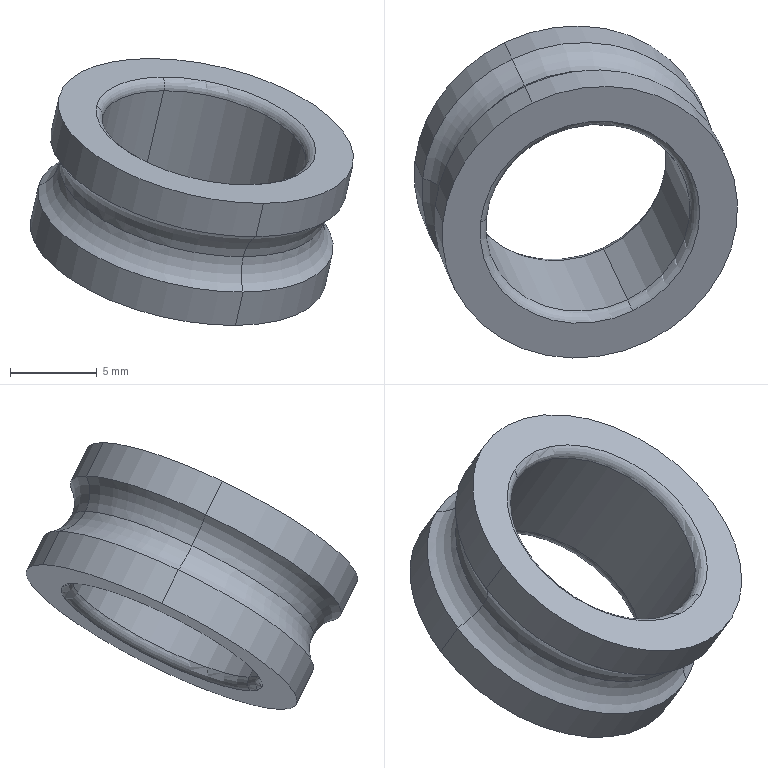Part | SolidWorks | features BaseBody 1 | 1 solid | 23 faces | box 18.588 x 19.086 x 15.342 mm | volume 855.538 mm3 | torus 12 | cylinder 9 | plane 2 | commonest cylinder face diameters 17.332 x6 12 x3
STEP:
#1=CARTESIAN_POINT('',(1933.787,-172.528,834.056));
#2=VERTEX_POINT('',#1);
#3=CARTESIAN_POINT('',(1934.502,-174.042,835.206));
#4=VERTEX_POINT('',#3);
#5=CARTESIAN_POINT('',(1934.646,-174.305,832.976));
#6=DIRECTION('',(0.9021,0.4315,0.007269));
#7=DIRECTION('',(-0.3816,0.7898,0.4803));
#8=AXIS2_PLACEMENT_3D('',#5,#6,#7);
#9=CIRCLE('',#8,2.25);
#10=EDGE_CURVE('',#2,#4,#9,.T.);
#11=ORIENTED_EDGE('',*,*,#10,.F.);
#12=CARTESIAN_POINT('',(1927.872,-160.287,841.5));
#13=VERTEX_POINT('',#12);
#14=CARTESIAN_POINT('',(1930.83,-166.408,837.778));
#15=DIRECTION('',(0.2015,-0.436,0.8771));
#16=DIRECTION('',(0.,-0.8955,-0.4451));
#17=AXIS2_PLACEMENT_3D('',#14,#15,#16);
#18=CIRCLE('',#17,7.75);
#19=EDGE_CURVE('',#2,#13,#18,.T.);
#20=ORIENTED_EDGE('',*,*,#19,.T.);
#21=CARTESIAN_POINT('',(1927.888,-160.353,843.529));
#22=VERTEX_POINT('',#21);
#23=CARTESIAN_POINT('',(1927.014,-158.51,842.581));
#24=DIRECTION('',(0.9021,0.4315,0.007269));
#25=DIRECTION('',(0.3816,-0.7898,-0.4803));
#26=AXIS2_PLACEMENT_3D('',#23,#24,#25);
#27=CIRCLE('',#26,2.25);
#28=EDGE_CURVE('',#22,#13,#27,.T.);
#29=ORIENTED_EDGE('',*,*,#28,.F.);
#30=CARTESIAN_POINT('',(1931.195,-167.198,839.367));
#31=DIRECTION('',(-0.2015,0.436,-0.8771));
#32=DIRECTION('',(-0.3816,0.7898,0.4803));
#33=AXIS2_PLACEMENT_3D('',#30,#31,#32);
#34=CIRCLE('',#33,8.666);
#35=EDGE_CURVE('',#22,#4,#34,.T.);
#36=ORIENTED_EDGE('',*,*,#35,.T.);
#37=EDGE_LOOP('',(#11,#20,#29,#36));
#38=FACE_OUTER_BOUND('',#37,.T.);
#39=CARTESIAN_POINT('',(1930.83,-166.408,837.778));
#40=DIRECTION('',(0.2015,-0.436,0.8771));
#41=DIRECTION('',(-0.9746,0.,0.2239));
#42=AXIS2_PLACEMENT_3D('',#39,#40,#41);
#43=TOROIDAL_SURFACE('',#42,10.,2.25);
#44=ADVANCED_FACE('',(#38),#43,.F.);
#45=ORIENTED_EDGE('',*,*,#28,.T.);
#46=CARTESIAN_POINT('',(1923.276,-166.408,839.513));
#47=VERTEX_POINT('',#46);
#48=CARTESIAN_POINT('',(1930.83,-166.408,837.778));
#49=DIRECTION('',(0.2015,-0.436,0.8771));
#50=DIRECTION('',(0.,-0.8955,-0.4451));
#51=AXIS2_PLACEMENT_3D('',#48,#49,#50);
#52=CIRCLE('',#51,7.75);
#53=EDGE_CURVE('',#13,#47,#52,.T.);
#54=ORIENTED_EDGE('',*,*,#53,.T.);
#55=CARTESIAN_POINT('',(1922.749,-167.198,841.307));
#56=VERTEX_POINT('',#55);
#57=CARTESIAN_POINT('',(1921.083,-166.408,840.017));
#58=DIRECTION('',(0.09761,0.8999,0.425));
#59=DIRECTION('',(0.,-0.427,0.9043));
#60=AXIS2_PLACEMENT_3D('',#57,#58,#59);
#61=CIRCLE('',#60,2.25);
#62=EDGE_CURVE('',#56,#47,#61,.T.);
#63=ORIENTED_EDGE('',*,*,#62,.F.);
#64=CARTESIAN_POINT('',(1931.195,-167.198,839.367));
#65=DIRECTION('',(-0.2015,0.436,-0.8771));
#66=DIRECTION('',(0.3816,-0.7898,-0.4803));
#67=AXIS2_PLACEMENT_3D('',#64,#65,#66);
#68=CIRCLE('',#67,8.666);
#69=EDGE_CURVE('',#56,#22,#68,.T.);
#70=ORIENTED_EDGE('',*,*,#69,.T.);
#71=EDGE_LOOP('',(#45,#54,#63,#70));
#72=FACE_OUTER_BOUND('',#71,.T.);
#73=CARTESIAN_POINT('',(1930.83,-166.408,837.778));
#74=DIRECTION('',(0.2015,-0.436,0.8771));
#75=DIRECTION('',(-0.9746,0.,0.2239));
#76=AXIS2_PLACEMENT_3D('',#73,#74,#75);
#77=TOROIDAL_SURFACE('',#76,10.,2.25);
#78=ADVANCED_FACE('',(#72),#77,.F.);
#79=ORIENTED_EDGE('',*,*,#62,.T.);
#80=CARTESIAN_POINT('',(1930.83,-166.408,837.778));
#81=DIRECTION('',(0.2015,-0.436,0.8771));
#82=DIRECTION('',(0.,-0.8955,-0.4451));
#83=AXIS2_PLACEMENT_3D('',#80,#81,#82);
#84=CIRCLE('',#83,7.75);
#85=EDGE_CURVE('',#47,#2,#84,.T.);
#86=ORIENTED_EDGE('',*,*,#85,.T.);
#87=ORIENTED_EDGE('',*,*,#10,.T.);
#88=CARTESIAN_POINT('',(1931.195,-167.198,839.367));
#89=DIRECTION('',(-0.2015,0.436,-0.8771));
#90=DIRECTION('',(0.3816,-0.7898,-0.4803));
#91=AXIS2_PLACEMENT_3D('',#88,#89,#90);
#92=CIRCLE('',#91,8.666);
#93=EDGE_CURVE('',#4,#56,#92,.T.);
#94=ORIENTED_EDGE('',*,*,#93,.T.);
#95=EDGE_LOOP('',(#79,#86,#87,#94));
#96=FACE_OUTER_BOUND('',#95,.T.);
#97=CARTESIAN_POINT('',(1930.83,-166.408,837.778));
#98=DIRECTION('',(0.2015,-0.436,0.8771));
#99=DIRECTION('',(-0.9746,0.,0.2239));
#100=AXIS2_PLACEMENT_3D('',#97,#98,#99);
#101=TOROIDAL_SURFACE('',#100,10.,2.25);
#102=ADVANCED_FACE('',(#96),#101,.F.);
#103=CARTESIAN_POINT('',(1927.865,-160.208,837.722));
#104=VERTEX_POINT('',#103);
#105=CARTESIAN_POINT('',(1924.307,-164.947,836.183));
#106=VERTEX_POINT('',#105);
#107=CARTESIAN_POINT('',(1930.155,-164.947,834.84));
#108=DIRECTION('',(0.2015,-0.436,0.8771));
#109=DIRECTION('',(-0.3816,0.7898,0.4803));
#110=AXIS2_PLACEMENT_3D('',#107,#108,#109);
#111=CIRCLE('',#110,6.);
#112=EDGE_CURVE('',#104,#106,#111,.T.);
#113=ORIENTED_EDGE('',*,*,#112,.T.);
#114=CARTESIAN_POINT('',(1923.737,-164.664,835.714));
#115=VERTEX_POINT('',#114);
#116=CARTESIAN_POINT('',(1923.63,-164.947,836.339));
#117=DIRECTION('',(0.09761,0.8999,0.425));
#118=DIRECTION('',(0.,-0.427,0.9043));
#119=AXIS2_PLACEMENT_3D('',#116,#117,#118);
#120=CIRCLE('',#119,0.6944);
#121=EDGE_CURVE('',#106,#115,#120,.T.);
#122=ORIENTED_EDGE('',*,*,#121,.T.);
#123=CARTESIAN_POINT('',(1927.562,-159.57,837.368));
#124=VERTEX_POINT('',#123);
#125=CARTESIAN_POINT('',(1930.024,-164.664,834.27));
#126=DIRECTION('',(0.2015,-0.436,0.8771));
#127=DIRECTION('',(-0.3816,0.7898,0.4803));
#128=AXIS2_PLACEMENT_3D('',#125,#126,#127);
#129=CIRCLE('',#128,6.45);
#130=EDGE_CURVE('',#124,#115,#129,.T.);
#131=ORIENTED_EDGE('',*,*,#130,.F.);
#132=CARTESIAN_POINT('',(1927.6,-159.66,838.055));
#133=DIRECTION('',(0.9021,0.4315,0.007269));
#134=DIRECTION('',(-0.05425,0.1301,-0.99));
#135=AXIS2_PLACEMENT_3D('',#132,#133,#134);
#136=CIRCLE('',#135,0.6944);
#137=EDGE_CURVE('',#104,#124,#136,.T.);
#138=ORIENTED_EDGE('',*,*,#137,.F.);
#139=EDGE_LOOP('',(#113,#122,#131,#138));
#140=FACE_OUTER_BOUND('',#139,.T.);
#141=CARTESIAN_POINT('',(1930.155,-164.947,834.84));
#142=DIRECTION('',(0.2015,-0.436,0.8771));
#143=DIRECTION('',(-0.9746,0.,0.2239));
#144=AXIS2_PLACEMENT_3D('',#141,#142,#143);
#145=TOROIDAL_SURFACE('',#144,6.694,0.6944);
#146=ADVANCED_FACE('',(#140),#145,.T.);
#147=CARTESIAN_POINT('',(1921.578,-164.664,836.21));
#148=VERTEX_POINT('',#147);
#149=CARTESIAN_POINT('',(1926.717,-157.819,838.432));
#150=VERTEX_POINT('',#149);
#151=CARTESIAN_POINT('',(1930.024,-164.664,834.27));
#152=DIRECTION('',(-0.2015,0.436,-0.8771));
#153=DIRECTION('',(0.3816,-0.7898,-0.4803));
#154=AXIS2_PLACEMENT_3D('',#151,#152,#153);
#155=CIRCLE('',#154,8.666);
#156=EDGE_CURVE('',#148,#150,#155,.T.);
#157=ORIENTED_EDGE('',*,*,#156,.F.);
#158=CARTESIAN_POINT('',(1922.019,-165.618,838.129));
#159=VERTEX_POINT('',#158);
#160=CARTESIAN_POINT('',(1921.566,-164.637,836.157));
#161=DIRECTION('',(0.2015,-0.436,0.8771));
#162=VECTOR('',#161,1000.);
#163=LINE('',#160,#162);
#164=EDGE_CURVE('',#148,#159,#163,.T.);
#165=ORIENTED_EDGE('',*,*,#164,.T.);
#166=CARTESIAN_POINT('',(1927.158,-158.773,840.351));
#167=VERTEX_POINT('',#166);
#168=CARTESIAN_POINT('',(1930.465,-165.618,836.189));
#169=DIRECTION('',(0.2015,-0.436,0.8771));
#170=DIRECTION('',(-0.3816,0.7898,0.4803));
#171=AXIS2_PLACEMENT_3D('',#168,#169,#170);
#172=CIRCLE('',#171,8.666);
#173=EDGE_CURVE('',#167,#159,#172,.T.);
#174=ORIENTED_EDGE('',*,*,#173,.F.);
#175=CARTESIAN_POINT('',(1927.158,-158.773,840.351));
#176=DIRECTION('',(0.2015,-0.436,0.8771));
#177=VECTOR('',#176,1000.);
#178=LINE('',#175,#177);
#179=EDGE_CURVE('',#150,#167,#178,.T.);
#180=ORIENTED_EDGE('',*,*,#179,.F.);
#181=EDGE_LOOP('',(#157,#165,#174,#180));
#182=FACE_OUTER_BOUND('',#181,.T.);
#183=CARTESIAN_POINT('',(1930.012,-164.637,834.217));
#184=DIRECTION('',(0.2015,-0.436,0.8771));
#185=DIRECTION('',(-0.9746,0.,0.2239));
#186=AXIS2_PLACEMENT_3D('',#183,#184,#185);
#187=CYLINDRICAL_SURFACE('',#186,8.666);
#188=ADVANCED_FACE('',(#182),#187,.T.);
#189=ORIENTED_EDGE('',*,*,#85,.F.);
#190=CARTESIAN_POINT('',(1921.083,-166.408,840.017));
#191=DIRECTION('',(0.09761,0.8999,0.425));
#192=DIRECTION('',(0.,-0.427,0.9043));
#193=AXIS2_PLACEMENT_3D('',#190,#191,#192);
#194=CIRCLE('',#193,2.25);
#195=EDGE_CURVE('',#47,#159,#194,.T.);
#196=ORIENTED_EDGE('',*,*,#195,.T.);
#197=CARTESIAN_POINT('',(1933.772,-172.462,832.027));
#198=VERTEX_POINT('',#197);
#199=CARTESIAN_POINT('',(1930.465,-165.618,836.189));
#200=DIRECTION('',(0.2015,-0.436,0.8771));
#201=DIRECTION('',(-0.3816,0.7898,0.4803));
#202=AXIS2_PLACEMENT_3D('',#199,#200,#201);
#203=CIRCLE('',#202,8.666);
#204=EDGE_CURVE('',#159,#198,#203,.T.);
#205=ORIENTED_EDGE('',*,*,#204,.T.);
#206=CARTESIAN_POINT('',(1934.646,-174.305,832.976));
#207=DIRECTION('',(0.9021,0.4315,0.007269));
#208=DIRECTION('',(-0.3816,0.7898,0.4803));
#209=AXIS2_PLACEMENT_3D('',#206,#207,#208);
#210=CIRCLE('',#209,2.25);
#211=EDGE_CURVE('',#198,#2,#210,.T.);
#212=ORIENTED_EDGE('',*,*,#211,.T.);
#213=EDGE_LOOP('',(#189,#196,#205,#212));
#214=FACE_OUTER_BOUND('',#213,.T.);
#215=CARTESIAN_POINT('',(1930.83,-166.408,837.778));
#216=DIRECTION('',(0.2015,-0.436,0.8771));
#217=DIRECTION('',(-0.9746,0.,0.2239));
#218=AXIS2_PLACEMENT_3D('',#215,#216,#217);
#219=TOROIDAL_SURFACE('',#218,10.,2.25);
#220=ADVANCED_FACE('',(#214),#219,.F.);
#221=ORIENTED_EDGE('',*,*,#69,.F.);
#222=CARTESIAN_POINT('',(1923.189,-168.152,843.227));
#223=VERTEX_POINT('',#222);
#224=CARTESIAN_POINT('',(1922.737,-167.171,841.255));
#225=DIRECTION('',(0.2015,-0.436,0.8771));
#226=VECTOR('',#225,1000.);
#227=LINE('',#224,#226);
#228=EDGE_CURVE('',#56,#223,#227,.T.);
#229=ORIENTED_EDGE('',*,*,#228,.T.);
#230=CARTESIAN_POINT('',(1928.329,-161.308,845.449));
#231=VERTEX_POINT('',#230);
#232=CARTESIAN_POINT('',(1931.636,-168.152,841.287));
#233=DIRECTION('',(0.2015,-0.436,0.8771));
#234=DIRECTION('',(-0.3816,0.7898,0.4803));
#235=AXIS2_PLACEMENT_3D('',#232,#233,#234);
#236=CIRCLE('',#235,8.666);
#237=EDGE_CURVE('',#231,#223,#236,.T.);
#238=ORIENTED_EDGE('',*,*,#237,.F.);
#239=CARTESIAN_POINT('',(1928.329,-161.308,845.449));
#240=DIRECTION('',(-0.2015,0.436,-0.8771));
#241=VECTOR('',#240,1000.);
#242=LINE('',#239,#241);
#243=EDGE_CURVE('',#231,#22,#242,.T.);
#244=ORIENTED_EDGE('',*,*,#243,.T.);
#245=EDGE_LOOP('',(#221,#229,#238,#244));
#246=FACE_OUTER_BOUND('',#245,.T.);
#247=CARTESIAN_POINT('',(1931.183,-167.171,839.315));
#248=DIRECTION('',(0.2015,-0.436,0.8771));
#249=DIRECTION('',(-0.9746,0.,0.2239));
#250=AXIS2_PLACEMENT_3D('',#247,#248,#249);
#251=CYLINDRICAL_SURFACE('',#250,8.666);
#252=ADVANCED_FACE('',(#246),#251,.T.);
#253=CARTESIAN_POINT('',(1925.349,-168.152,842.731));
#254=VERTEX_POINT('',#253);
#255=CARTESIAN_POINT('',(1929.174,-163.058,844.384));
#256=VERTEX_POINT('',#255);
#257=CARTESIAN_POINT('',(1931.636,-168.152,841.287));
#258=DIRECTION('',(-0.2015,0.436,-0.8771));
#259=DIRECTION('',(0.3816,-0.7898,-0.4803));
#260=AXIS2_PLACEMENT_3D('',#257,#258,#259);
#261=CIRCLE('',#260,6.45);
#262=EDGE_CURVE('',#254,#256,#261,.T.);
#263=ORIENTED_EDGE('',*,*,#262,.F.);
#264=CARTESIAN_POINT('',(1925.657,-167.868,842.06));
#265=VERTEX_POINT('',#264);
#266=CARTESIAN_POINT('',(1924.98,-167.868,842.215));
#267=DIRECTION('',(0.09761,0.8999,0.425));
#268=DIRECTION('',(0.,-0.427,0.9043));
#269=AXIS2_PLACEMENT_3D('',#266,#267,#268);
#270=CIRCLE('',#269,0.6944);
#271=EDGE_CURVE('',#254,#265,#270,.T.);
#272=ORIENTED_EDGE('',*,*,#271,.T.);
#273=CARTESIAN_POINT('',(1929.215,-163.13,843.598));
#274=VERTEX_POINT('',#273);
#275=CARTESIAN_POINT('',(1931.505,-167.868,840.717));
#276=DIRECTION('',(-0.2015,0.436,-0.8771));
#277=DIRECTION('',(0.3816,-0.7898,-0.4803));
#278=AXIS2_PLACEMENT_3D('',#275,#276,#277);
#279=CIRCLE('',#278,6.);
#280=EDGE_CURVE('',#265,#274,#279,.T.);
#281=ORIENTED_EDGE('',*,*,#280,.T.);
#282=CARTESIAN_POINT('',(1928.95,-162.581,843.932));
#283=DIRECTION('',(-0.9021,-0.4315,-0.007269));
#284=DIRECTION('',(0.3816,-0.7898,-0.4803));
#285=AXIS2_PLACEMENT_3D('',#282,#283,#284);
#286=CIRCLE('',#285,0.6944);
#287=EDGE_CURVE('',#274,#256,#286,.T.);
#288=ORIENTED_EDGE('',*,*,#287,.T.);
#289=EDGE_LOOP('',(#263,#272,#281,#288));
#290=FACE_OUTER_BOUND('',#289,.T.);
#291=CARTESIAN_POINT('',(1931.505,-167.868,840.717));
#292=DIRECTION('',(0.2015,-0.436,0.8771));
#293=DIRECTION('',(-0.9746,0.,0.2239));
#294=AXIS2_PLACEMENT_3D('',#291,#292,#293);
#295=TOROIDAL_SURFACE('',#294,6.694,0.6944);
#296=ADVANCED_FACE('',(#290),#295,.T.);
#297=CARTESIAN_POINT('',(1932.444,-169.686,831.958));
#298=VERTEX_POINT('',#297);
#299=CARTESIAN_POINT('',(1930.155,-164.947,834.84));
#300=DIRECTION('',(0.2015,-0.436,0.8771));
#301=DIRECTION('',(-0.3816,0.7898,0.4803));
#302=AXIS2_PLACEMENT_3D('',#299,#300,#301);
#303=CIRCLE('',#302,6.);
#304=EDGE_CURVE('',#106,#298,#303,.T.);
#305=ORIENTED_EDGE('',*,*,#304,.F.);
#306=CARTESIAN_POINT('',(1924.28,-164.889,836.066));
#307=DIRECTION('',(0.2015,-0.436,0.8771));
#308=VECTOR('',#307,1000.);
#309=LINE('',#306,#308);
#310=EDGE_CURVE('',#106,#265,#309,.T.);
#311=ORIENTED_EDGE('',*,*,#310,.T.);
#312=CARTESIAN_POINT('',(1933.794,-172.607,837.835));
#313=VERTEX_POINT('',#312);
#314=CARTESIAN_POINT('',(1931.505,-167.868,840.717));
#315=DIRECTION('',(-0.2015,0.436,-0.8771));
#316=DIRECTION('',(0.3816,-0.7898,-0.4803));
#317=AXIS2_PLACEMENT_3D('',#314,#315,#316);
#318=CIRCLE('',#317,6.);
#319=EDGE_CURVE('',#313,#265,#318,.T.);
#320=ORIENTED_EDGE('',*,*,#319,.F.);
#321=CARTESIAN_POINT('',(1932.444,-169.686,831.958));
#322=DIRECTION('',(-0.2015,0.436,-0.8771));
#323=VECTOR('',#322,1000.);
#324=LINE('',#321,#323);
#325=EDGE_CURVE('',#313,#298,#324,.T.);
#326=ORIENTED_EDGE('',*,*,#325,.T.);
#327=EDGE_LOOP('',(#305,#311,#320,#326));
#328=FACE_OUTER_BOUND('',#327,.T.);
#329=CARTESIAN_POINT('',(1930.128,-164.889,834.722));
#330=DIRECTION('',(0.2015,-0.436,0.8771));
#331=DIRECTION('',(-0.9746,0.,0.2239));
#332=AXIS2_PLACEMENT_3D('',#329,#330,#331);
#333=CYLINDRICAL_SURFACE('',#332,6.);
#334=ADVANCED_FACE('',(#328),#333,.F.);
#335=CARTESIAN_POINT('',(1930.155,-164.947,834.84));
#336=DIRECTION('',(0.2015,-0.436,0.8771));
#337=DIRECTION('',(0.3816,-0.7898,-0.4803));
#338=AXIS2_PLACEMENT_3D('',#335,#336,#337);
#339=CIRCLE('',#338,6.);
#340=EDGE_CURVE('',#298,#104,#339,.T.);
#341=ORIENTED_EDGE('',*,*,#340,.F.);
#342=ORIENTED_EDGE('',*,*,#325,.F.);
#343=CARTESIAN_POINT('',(1931.505,-167.868,840.717));
#344=DIRECTION('',(-0.2015,0.436,-0.8771));
#345=DIRECTION('',(-0.3816,0.7898,0.4803));
#346=AXIS2_PLACEMENT_3D('',#343,#344,#345);
#347=CIRCLE('',#346,6.);
#348=EDGE_CURVE('',#274,#313,#347,.T.);
#349=ORIENTED_EDGE('',*,*,#348,.F.);
#350=CARTESIAN_POINT('',(1927.865,-160.208,837.722));
#351=DIRECTION('',(0.2015,-0.436,0.8771));
#352=VECTOR('',#351,1000.);
#353=LINE('',#350,#352);
#354=EDGE_CURVE('',#104,#274,#353,.T.);
#355=ORIENTED_EDGE('',*,*,#354,.F.);
#356=EDGE_LOOP('',(#341,#342,#349,#355));
#357=FACE_OUTER_BOUND('',#356,.T.);
#358=CARTESIAN_POINT('',(1930.128,-164.889,834.722));
#359=DIRECTION('',(0.2015,-0.436,0.8771));
#360=DIRECTION('',(-0.9746,0.,0.2239));
#361=AXIS2_PLACEMENT_3D('',#358,#359,#360);
#362=CYLINDRICAL_SURFACE('',#361,6.);
#363=ADVANCED_FACE('',(#357),#362,.F.);
#364=ORIENTED_EDGE('',*,*,#310,.F.);
#365=ORIENTED_EDGE('',*,*,#112,.F.);
#366=ORIENTED_EDGE('',*,*,#354,.T.);
#367=ORIENTED_EDGE('',*,*,#280,.F.);
#368=EDGE_LOOP('',(#364,#365,#366,#367));
#369=FACE_OUTER_BOUND('',#368,.T.);
#370=CARTESIAN_POINT('',(1930.128,-164.889,834.722));
#371=DIRECTION('',(0.2015,-0.436,0.8771));
#372=DIRECTION('',(-0.9746,0.,0.2239));
#373=AXIS2_PLACEMENT_3D('',#370,#371,#372);
#374=CYLINDRICAL_SURFACE('',#373,6.);
#375=ADVANCED_FACE('',(#369),#374,.F.);
#376=ORIENTED_EDGE('',*,*,#271,.F.);
#377=CARTESIAN_POINT('',(1934.097,-173.246,838.189));
#378=VERTEX_POINT('',#377);
#379=CARTESIAN_POINT('',(1931.636,-168.152,841.287));
#380=DIRECTION('',(-0.2015,0.436,-0.8771));
#381=DIRECTION('',(0.3816,-0.7898,-0.4803));
#382=AXIS2_PLACEMENT_3D('',#379,#380,#381);
#383=CIRCLE('',#382,6.45);
#384=EDGE_CURVE('',#378,#254,#383,.T.);
#385=ORIENTED_EDGE('',*,*,#384,.F.);
#386=CARTESIAN_POINT('',(1934.059,-173.155,837.501));
#387=DIRECTION('',(-0.9021,-0.4315,-0.007269));
#388=DIRECTION('',(-0.3816,0.7898,0.4803));
#389=AXIS2_PLACEMENT_3D('',#386,#387,#388);
#390=CIRCLE('',#389,0.6944);
#391=EDGE_CURVE('',#378,#313,#390,.T.);
#392=ORIENTED_EDGE('',*,*,#391,.T.);
#393=ORIENTED_EDGE('',*,*,#319,.T.);
#394=EDGE_LOOP('',(#376,#385,#392,#393));
#395=FACE_OUTER_BOUND('',#394,.T.);
#396=CARTESIAN_POINT('',(1931.505,-167.868,840.717));
#397=DIRECTION('',(0.2015,-0.436,0.8771));
#398=DIRECTION('',(-0.9746,0.,0.2239));
#399=AXIS2_PLACEMENT_3D('',#396,#397,#398);
#400=TOROIDAL_SURFACE('',#399,6.694,0.6944);
#401=ADVANCED_FACE('',(#395),#400,.T.);
#402=ORIENTED_EDGE('',*,*,#348,.T.);
#403=ORIENTED_EDGE('',*,*,#391,.F.);
#404=CARTESIAN_POINT('',(1931.636,-168.152,841.287));
#405=DIRECTION('',(-0.2015,0.436,-0.8771));
#406=DIRECTION('',(-0.3816,0.7898,0.4803));
#407=AXIS2_PLACEMENT_3D('',#404,#405,#406);
#408=CIRCLE('',#407,6.45);
#409=EDGE_CURVE('',#256,#378,#408,.T.);
#410=ORIENTED_EDGE('',*,*,#409,.F.);
#411=ORIENTED_EDGE('',*,*,#287,.F.);
#412=EDGE_LOOP('',(#402,#403,#410,#411));
#413=FACE_OUTER_BOUND('',#412,.T.);
#414=CARTESIAN_POINT('',(1931.505,-167.868,840.717));
#415=DIRECTION('',(0.2015,-0.436,0.8771));
#416=DIRECTION('',(-0.9746,0.,0.2239));
#417=AXIS2_PLACEMENT_3D('',#414,#415,#416);
#418=TOROIDAL_SURFACE('',#417,6.694,0.6944);
#419=ADVANCED_FACE('',(#413),#418,.T.);
#420=CARTESIAN_POINT('',(1934.942,-174.996,837.125));
#421=VERTEX_POINT('',#420);
#422=CARTESIAN_POINT('',(1931.636,-168.152,841.287));
#423=DIRECTION('',(0.2015,-0.436,0.8771));
#424=DIRECTION('',(0.3816,-0.7898,-0.4803));
#425=AXIS2_PLACEMENT_3D('',#422,#423,#424);
#426=CIRCLE('',#425,8.666);
#427=EDGE_CURVE('',#421,#231,#426,.T.);
#428=ORIENTED_EDGE('',*,*,#427,.T.);
#429=ORIENTED_EDGE('',*,*,#237,.T.);
#430=CARTESIAN_POINT('',(1931.636,-168.152,841.287));
#431=DIRECTION('',(0.2015,-0.436,0.8771));
#432=DIRECTION('',(-0.3816,0.7898,0.4803));
#433=AXIS2_PLACEMENT_3D('',#430,#431,#432);
#434=CIRCLE('',#433,8.666);
#435=EDGE_CURVE('',#223,#421,#434,.T.);
#436=ORIENTED_EDGE('',*,*,#435,.T.);
#437=EDGE_LOOP('',(#428,#429,#436));
#438=FACE_OUTER_BOUND('',#437,.T.);
#439=ORIENTED_EDGE('',*,*,#409,.T.);
#440=ORIENTED_EDGE('',*,*,#384,.T.);
#441=ORIENTED_EDGE('',*,*,#262,.T.);
#442=EDGE_LOOP('',(#439,#440,#441));
#443=FACE_BOUND('',#442,.T.);
#444=CARTESIAN_POINT('',(1923.731,-160.041,847.134));
#445=DIRECTION('',(0.2015,-0.436,0.8771));
#446=DIRECTION('',(-0.09761,-0.8999,-0.425));
#447=AXIS2_PLACEMENT_3D('',#444,#445,#446);
#448=PLANE('',#447);
#449=ADVANCED_FACE('',(#438,#443),#448,.T.);
#450=ORIENTED_EDGE('',*,*,#243,.F.);
#451=ORIENTED_EDGE('',*,*,#427,.F.);
#452=CARTESIAN_POINT('',(1934.942,-174.996,837.125));
#453=DIRECTION('',(0.2015,-0.436,0.8771));
#454=VECTOR('',#453,1000.);
#455=LINE('',#452,#454);
#456=EDGE_CURVE('',#4,#421,#455,.T.);
#457=ORIENTED_EDGE('',*,*,#456,.F.);
#458=ORIENTED_EDGE('',*,*,#35,.F.);
#459=EDGE_LOOP('',(#450,#451,#457,#458));
#460=FACE_OUTER_BOUND('',#459,.T.);
#461=CARTESIAN_POINT('',(1931.183,-167.171,839.315));
#462=DIRECTION('',(0.2015,-0.436,0.8771));
#463=DIRECTION('',(-0.9746,0.,0.2239));
#464=AXIS2_PLACEMENT_3D('',#461,#462,#463);
#465=CYLINDRICAL_SURFACE('',#464,8.666);
#466=ADVANCED_FACE('',(#460),#465,.T.);
#467=ORIENTED_EDGE('',*,*,#228,.F.);
#468=ORIENTED_EDGE('',*,*,#93,.F.);
#469=ORIENTED_EDGE('',*,*,#456,.T.);
#470=ORIENTED_EDGE('',*,*,#435,.F.);
#471=EDGE_LOOP('',(#467,#468,#469,#470));
#472=FACE_OUTER_BOUND('',#471,.T.);
#473=CARTESIAN_POINT('',(1931.183,-167.171,839.315));
#474=DIRECTION('',(0.2015,-0.436,0.8771));
#475=DIRECTION('',(-0.9746,0.,0.2239));
#476=AXIS2_PLACEMENT_3D('',#473,#474,#475);
#477=CYLINDRICAL_SURFACE('',#476,8.666);
#478=ADVANCED_FACE('',(#472),#477,.T.);
#479=ORIENTED_EDGE('',*,*,#53,.F.);
#480=CARTESIAN_POINT('',(1927.014,-158.51,842.581));
#481=DIRECTION('',(0.9021,0.4315,0.007269));
#482=DIRECTION('',(0.3816,-0.7898,-0.4803));
#483=AXIS2_PLACEMENT_3D('',#480,#481,#482);
#484=CIRCLE('',#483,2.25);
#485=EDGE_CURVE('',#13,#167,#484,.T.);
#486=ORIENTED_EDGE('',*,*,#485,.T.);
#487=ORIENTED_EDGE('',*,*,#173,.T.);
#488=ORIENTED_EDGE('',*,*,#195,.F.);
#489=EDGE_LOOP('',(#479,#486,#487,#488));
#490=FACE_OUTER_BOUND('',#489,.T.);
#491=CARTESIAN_POINT('',(1930.83,-166.408,837.778));
#492=DIRECTION('',(0.2015,-0.436,0.8771));
#493=DIRECTION('',(-0.9746,0.,0.2239));
#494=AXIS2_PLACEMENT_3D('',#491,#492,#493);
#495=TOROIDAL_SURFACE('',#494,10.,2.25);
#496=ADVANCED_FACE('',(#490),#495,.F.);
#497=ORIENTED_EDGE('',*,*,#19,.F.);
#498=ORIENTED_EDGE('',*,*,#211,.F.);
#499=CARTESIAN_POINT('',(1930.465,-165.618,836.189));
#500=DIRECTION('',(0.2015,-0.436,0.8771));
#501=DIRECTION('',(0.3816,-0.7898,-0.4803));
#502=AXIS2_PLACEMENT_3D('',#499,#500,#501);
#503=CIRCLE('',#502,8.666);
#504=EDGE_CURVE('',#198,#167,#503,.T.);
#505=ORIENTED_EDGE('',*,*,#504,.T.);
#506=ORIENTED_EDGE('',*,*,#485,.F.);
#507=EDGE_LOOP('',(#497,#498,#505,#506));
#508=FACE_OUTER_BOUND('',#507,.T.);
#509=CARTESIAN_POINT('',(1930.83,-166.408,837.778));
#510=DIRECTION('',(0.2015,-0.436,0.8771));
#511=DIRECTION('',(-0.9746,0.,0.2239));
#512=AXIS2_PLACEMENT_3D('',#509,#510,#511);
#513=TOROIDAL_SURFACE('',#512,10.,2.25);
#514=ADVANCED_FACE('',(#508),#513,.F.);
#515=ORIENTED_EDGE('',*,*,#504,.F.);
#516=CARTESIAN_POINT('',(1933.331,-171.508,830.108));
#517=VERTEX_POINT('',#516);
#518=CARTESIAN_POINT('',(1933.772,-172.462,832.027));
#519=DIRECTION('',(-0.2015,0.436,-0.8771));
#520=VECTOR('',#519,1000.);
#521=LINE('',#518,#520);
#522=EDGE_CURVE('',#198,#517,#521,.T.);
#523=ORIENTED_EDGE('',*,*,#522,.T.);
#524=CARTESIAN_POINT('',(1930.024,-164.664,834.27));
#525=DIRECTION('',(-0.2015,0.436,-0.8771));
#526=DIRECTION('',(-0.3816,0.7898,0.4803));
#527=AXIS2_PLACEMENT_3D('',#524,#525,#526);
#528=CIRCLE('',#527,8.666);
#529=EDGE_CURVE('',#150,#517,#528,.T.);
#530=ORIENTED_EDGE('',*,*,#529,.F.);
#531=ORIENTED_EDGE('',*,*,#179,.T.);
#532=EDGE_LOOP('',(#515,#523,#530,#531));
#533=FACE_OUTER_BOUND('',#532,.T.);
#534=CARTESIAN_POINT('',(1930.012,-164.637,834.217));
#535=DIRECTION('',(0.2015,-0.436,0.8771));
#536=DIRECTION('',(-0.9746,0.,0.2239));
#537=AXIS2_PLACEMENT_3D('',#534,#535,#536);
#538=CYLINDRICAL_SURFACE('',#537,8.666);
#539=ADVANCED_FACE('',(#533),#538,.T.);
#540=ORIENTED_EDGE('',*,*,#164,.F.);
#541=CARTESIAN_POINT('',(1930.024,-164.664,834.27));
#542=DIRECTION('',(-0.2015,0.436,-0.8771));
#543=DIRECTION('',(0.3816,-0.7898,-0.4803));
#544=AXIS2_PLACEMENT_3D('',#541,#542,#543);
#545=CIRCLE('',#544,8.666);
#546=EDGE_CURVE('',#517,#148,#545,.T.);
#547=ORIENTED_EDGE('',*,*,#546,.F.);
#548=ORIENTED_EDGE('',*,*,#522,.F.);
#549=ORIENTED_EDGE('',*,*,#204,.F.);
#550=EDGE_LOOP('',(#540,#547,#548,#549));
#551=FACE_OUTER_BOUND('',#550,.T.);
#552=CARTESIAN_POINT('',(1930.012,-164.637,834.217));
#553=DIRECTION('',(0.2015,-0.436,0.8771));
#554=DIRECTION('',(-0.9746,0.,0.2239));
#555=AXIS2_PLACEMENT_3D('',#552,#553,#554);
#556=CYLINDRICAL_SURFACE('',#555,8.666);
#557=ADVANCED_FACE('',(#551),#556,.T.);
#558=ORIENTED_EDGE('',*,*,#529,.T.);
#559=ORIENTED_EDGE('',*,*,#546,.T.);
#560=ORIENTED_EDGE('',*,*,#156,.T.);
#561=EDGE_LOOP('',(#558,#559,#560));
#562=FACE_OUTER_BOUND('',#561,.T.);
#563=CARTESIAN_POINT('',(1932.485,-169.758,831.172));
#564=VERTEX_POINT('',#563);
#565=CARTESIAN_POINT('',(1930.024,-164.664,834.27));
#566=DIRECTION('',(0.2015,-0.436,0.8771));
#567=DIRECTION('',(0.3816,-0.7898,-0.4803));
#568=AXIS2_PLACEMENT_3D('',#565,#566,#567);
#569=CIRCLE('',#568,6.45);
#570=EDGE_CURVE('',#564,#124,#569,.T.);
#571=ORIENTED_EDGE('',*,*,#570,.T.);
#572=ORIENTED_EDGE('',*,*,#130,.T.);
#573=CARTESIAN_POINT('',(1930.024,-164.664,834.27));
#574=DIRECTION('',(0.2015,-0.436,0.8771));
#575=DIRECTION('',(-0.3816,0.7898,0.4803));
#576=AXIS2_PLACEMENT_3D('',#573,#574,#575);
#577=CIRCLE('',#576,6.45);
#578=EDGE_CURVE('',#115,#564,#577,.T.);
#579=ORIENTED_EDGE('',*,*,#578,.T.);
#580=EDGE_LOOP('',(#571,#572,#579));
#581=FACE_BOUND('',#580,.T.);
#582=CARTESIAN_POINT('',(1922.119,-156.552,840.118));
#583=DIRECTION('',(-0.2015,0.436,-0.8771));
#584=DIRECTION('',(0.9746,0.,-0.2239));
#585=AXIS2_PLACEMENT_3D('',#582,#583,#584);
#586=PLANE('',#585);
#587=ADVANCED_FACE('',(#562,#581),#586,.T.);
#588=ORIENTED_EDGE('',*,*,#137,.T.);
#589=ORIENTED_EDGE('',*,*,#570,.F.);
#590=CARTESIAN_POINT('',(1932.709,-170.234,831.625));
#591=DIRECTION('',(0.9021,0.4315,0.007269));
#592=DIRECTION('',(-0.3229,0.6861,-0.6519));
#593=AXIS2_PLACEMENT_3D('',#590,#591,#592);
#594=CIRCLE('',#593,0.6944);
#595=EDGE_CURVE('',#564,#298,#594,.T.);
#596=ORIENTED_EDGE('',*,*,#595,.T.);
#597=ORIENTED_EDGE('',*,*,#340,.T.);
#598=EDGE_LOOP('',(#588,#589,#596,#597));
#599=FACE_OUTER_BOUND('',#598,.T.);
#600=CARTESIAN_POINT('',(1930.155,-164.947,834.84));
#601=DIRECTION('',(0.2015,-0.436,0.8771));
#602=DIRECTION('',(-0.9746,0.,0.2239));
#603=AXIS2_PLACEMENT_3D('',#600,#601,#602);
#604=TOROIDAL_SURFACE('',#603,6.694,0.6944);
#605=ADVANCED_FACE('',(#599),#604,.T.);
#606=ORIENTED_EDGE('',*,*,#121,.F.);
#607=ORIENTED_EDGE('',*,*,#304,.T.);
#608=ORIENTED_EDGE('',*,*,#595,.F.);
#609=ORIENTED_EDGE('',*,*,#578,.F.);
#610=EDGE_LOOP('',(#606,#607,#608,#609));
#611=FACE_OUTER_BOUND('',#610,.T.);
#612=CARTESIAN_POINT('',(1930.155,-164.947,834.84));
#613=DIRECTION('',(0.2015,-0.436,0.8771));
#614=DIRECTION('',(-0.9746,0.,0.2239));
#615=AXIS2_PLACEMENT_3D('',#612,#613,#614);
#616=TOROIDAL_SURFACE('',#615,6.694,0.6944);
#617=ADVANCED_FACE('',(#611),#616,.T.);
#618=CLOSED_SHELL('',(#44,#78,#102,#146,#188,#220,#252,#296,#334,#363,#375,#401,#419,#449,#466,#478,#496,#514,#539,#557,#587,#605,#617));
#619=MANIFOLD_SOLID_BREP('',#618);
#620=CARTESIAN_POINT('',(0.,0.,0.));
#621=DIRECTION('',(0.,0.,1.));
#622=DIRECTION('',(1.,0.,0.));
#623=AXIS2_PLACEMENT_3D('',#620,#621,#622);
#624=(LENGTH_UNIT()NAMED_UNIT(*)SI_UNIT(.MILLI.,.METRE.));
#625=UNCERTAINTY_MEASURE_WITH_UNIT(LENGTH_MEASURE(0.00001),#624,'','');
#626=(NAMED_UNIT(*)PLANE_ANGLE_UNIT()SI_UNIT($,.RADIAN.));
#627=(NAMED_UNIT(*)SI_UNIT($,.STERADIAN.)SOLID_ANGLE_UNIT());
#628=(GEOMETRIC_REPRESENTATION_CONTEXT(3)GLOBAL_UNCERTAINTY_ASSIGNED_CONTEXT((#625))GLOBAL_UNIT_ASSIGNED_CONTEXT((#624,#626,#627))REPRESENTATION_CONTEXT('',''));
#629=ADVANCED_BREP_SHAPE_REPRESENTATION('',(#619,#623),#628);